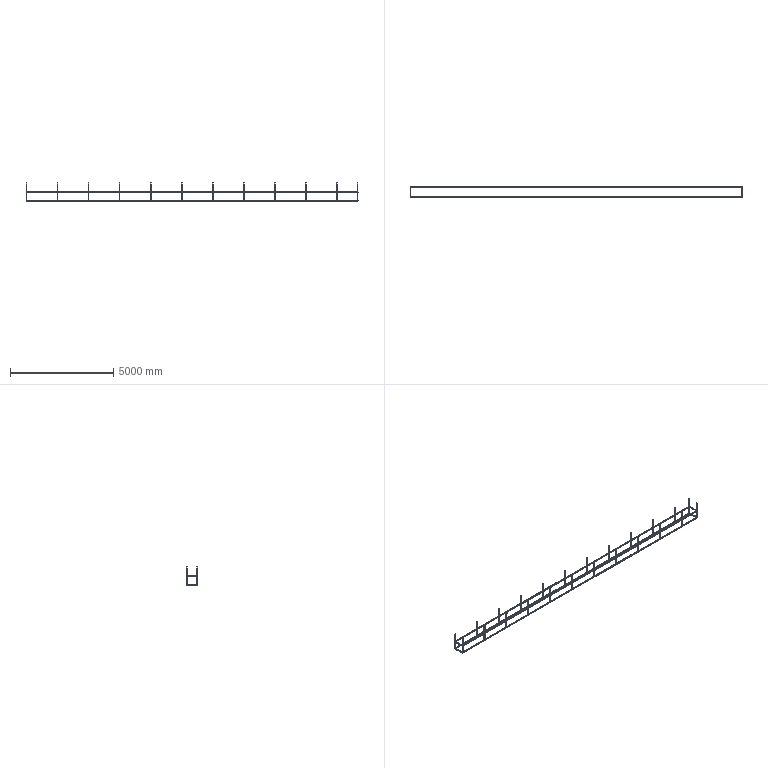Part | SolidWorks | features LPattern 2, 3DProfileFeature 1, WeldMemberFeat 1, WeldmentFeature 1 | 32 solids | 5888 faces | volume 48717671 mm3 | plane 3392 | cylinder 2496 | commonest cylinder face diameters 0.6 x1280 2 x896 5.8 x128 9 x128 6.8 x64